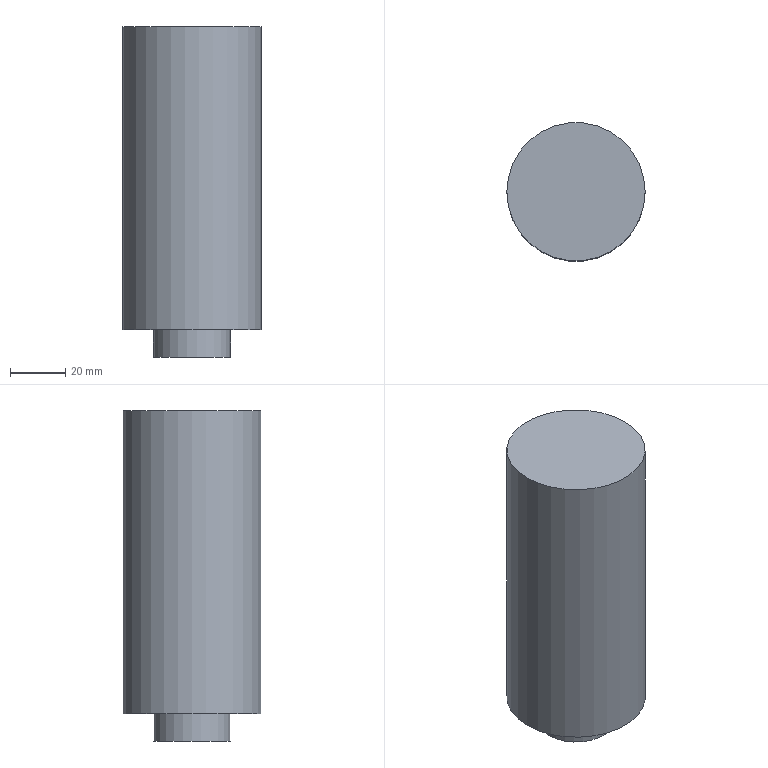Part | NX | features MAIN_BODY 2 | 1 solid | 5 faces | box 50.2 x 50.2 x 120 mm | volume 223873 mm3 | plane 3 | cylinder 2 | commonest cylinder face diameters 28 x1 50.2 x1
STEP:
#1=CARTESIAN_POINT('',(-64.9,255.,330.));
#2=VERTEX_POINT('',#1);
#3=CARTESIAN_POINT('',(-90.,255.,330.));
#4=DIRECTION('',(0.,0.,1.));
#5=DIRECTION('',(1.,0.,0.));
#6=AXIS2_PLACEMENT_3D('',#3,#4,#5);
#7=CIRCLE('',#6,25.1);
#8=EDGE_CURVE('',#2,#2,#7,.T.);
#9=ORIENTED_EDGE('',*,*,#8,.T.);
#10=EDGE_LOOP('',(#9));
#11=FACE_BOUND('',#10,.T.);
#12=CARTESIAN_POINT('',(-90.,264.25,330.));
#13=DIRECTION('',(0.,0.,1.));
#14=DIRECTION('',(1.,0.,0.));
#15=AXIS2_PLACEMENT_3D('',#12,#13,#14);
#16=PLANE('',#15);
#17=ADVANCED_FACE('',(#11),#16,.T.);
#18=ORIENTED_EDGE('',*,*,#8,.F.);
#19=EDGE_LOOP('',(#18));
#20=FACE_BOUND('',#19,.T.);
#21=CARTESIAN_POINT('',(-64.9,255.,220.));
#22=VERTEX_POINT('',#21);
#23=CARTESIAN_POINT('',(-90.,255.,220.));
#24=DIRECTION('',(0.,0.,1.));
#25=DIRECTION('',(1.,0.,0.));
#26=AXIS2_PLACEMENT_3D('',#23,#24,#25);
#27=CIRCLE('',#26,25.1);
#28=EDGE_CURVE('',#22,#22,#27,.T.);
#29=ORIENTED_EDGE('',*,*,#28,.T.);
#30=EDGE_LOOP('',(#29));
#31=FACE_BOUND('',#30,.T.);
#32=CARTESIAN_POINT('',(-90.,255.,330.));
#33=DIRECTION('',(0.,0.,-1.));
#34=DIRECTION('',(1.,0.,0.));
#35=AXIS2_PLACEMENT_3D('',#32,#33,#34);
#36=CYLINDRICAL_SURFACE('',#35,25.1);
#37=ADVANCED_FACE('',(#20,#31),#36,.T.);
#38=CARTESIAN_POINT('',(-76.,255.,220.));
#39=VERTEX_POINT('',#38);
#40=CARTESIAN_POINT('',(-90.,255.,220.));
#41=DIRECTION('',(0.,0.,1.));
#42=DIRECTION('',(1.,0.,0.));
#43=AXIS2_PLACEMENT_3D('',#40,#41,#42);
#44=CIRCLE('',#43,14.);
#45=EDGE_CURVE('',#39,#39,#44,.T.);
#46=ORIENTED_EDGE('',*,*,#45,.T.);
#47=EDGE_LOOP('',(#46));
#48=FACE_BOUND('',#47,.T.);
#49=ORIENTED_EDGE('',*,*,#28,.F.);
#50=EDGE_LOOP('',(#49));
#51=FACE_BOUND('',#50,.T.);
#52=CARTESIAN_POINT('',(-90.,264.25,220.));
#53=DIRECTION('',(0.,0.,-1.));
#54=DIRECTION('',(0.,1.,0.));
#55=AXIS2_PLACEMENT_3D('',#52,#53,#54);
#56=PLANE('',#55);
#57=ADVANCED_FACE('',(#48,#51),#56,.T.);
#58=ORIENTED_EDGE('',*,*,#45,.F.);
#59=EDGE_LOOP('',(#58));
#60=FACE_BOUND('',#59,.T.);
#61=CARTESIAN_POINT('',(-104.,255.,210.));
#62=VERTEX_POINT('',#61);
#63=CARTESIAN_POINT('',(-90.,255.,210.));
#64=DIRECTION('',(0.,0.,-1.));
#65=DIRECTION('',(-1.,0.,0.));
#66=AXIS2_PLACEMENT_3D('',#63,#64,#65);
#67=CIRCLE('',#66,14.);
#68=EDGE_CURVE('',#62,#62,#67,.F.);
#69=ORIENTED_EDGE('',*,*,#68,.T.);
#70=EDGE_LOOP('',(#69));
#71=FACE_BOUND('',#70,.T.);
#72=CARTESIAN_POINT('',(-90.,255.,202.26));
#73=DIRECTION('',(0.,0.,-1.));
#74=DIRECTION('',(0.,1.,0.));
#75=AXIS2_PLACEMENT_3D('',#72,#73,#74);
#76=CYLINDRICAL_SURFACE('',#75,14.);
#77=ADVANCED_FACE('',(#60,#71),#76,.T.);
#78=ORIENTED_EDGE('',*,*,#68,.F.);
#79=EDGE_LOOP('',(#78));
#80=FACE_BOUND('',#79,.T.);
#81=CARTESIAN_POINT('',(-90.,259.348,210.));
#82=DIRECTION('',(0.,0.,-1.));
#83=DIRECTION('',(0.,1.,0.));
#84=AXIS2_PLACEMENT_3D('',#81,#82,#83);
#85=PLANE('',#84);
#86=ADVANCED_FACE('',(#80),#85,.T.);
#87=CLOSED_SHELL('',(#17,#37,#57,#77,#86));
#88=MANIFOLD_SOLID_BREP('',#87);
#89=(LENGTH_UNIT()NAMED_UNIT(*)SI_UNIT(.MILLI.,.METRE.));
#90=UNCERTAINTY_MEASURE_WITH_UNIT(LENGTH_MEASURE(0.00001),#89,'','');
#91=(NAMED_UNIT(*)PLANE_ANGLE_UNIT()SI_UNIT($,.RADIAN.));
#92=(NAMED_UNIT(*)SI_UNIT($,.STERADIAN.)SOLID_ANGLE_UNIT());
#93=(GEOMETRIC_REPRESENTATION_CONTEXT(3)GLOBAL_UNCERTAINTY_ASSIGNED_CONTEXT((#90))GLOBAL_UNIT_ASSIGNED_CONTEXT((#89,#91,#92))REPRESENTATION_CONTEXT('',''));
#94=ADVANCED_BREP_SHAPE_REPRESENTATION('',(#88),#93);